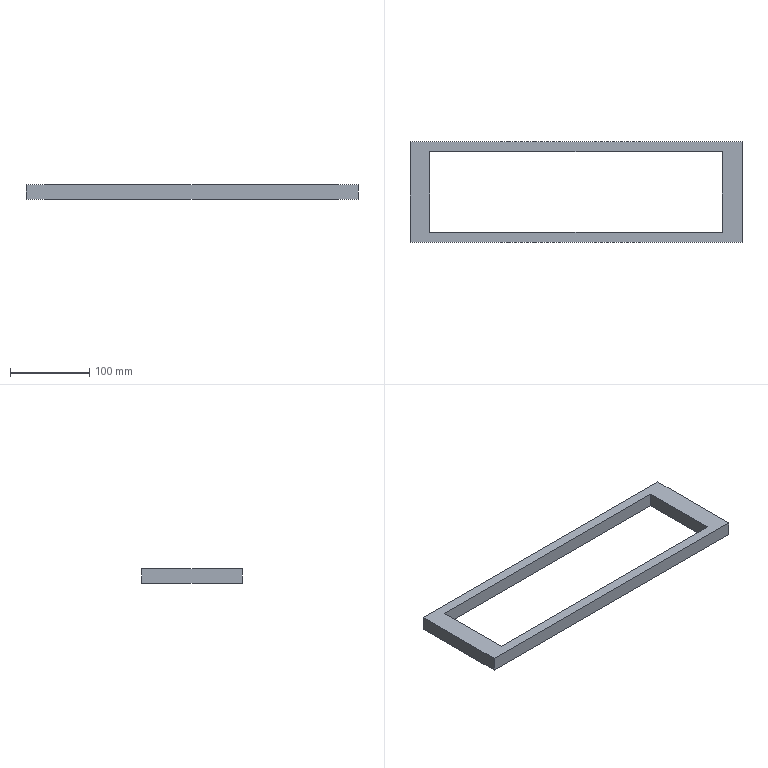Part | SolidWorks | features Extrusion 1 | 1 solid | 10 faces | box 420 x 127 x 18 mm | volume 280800 mm3 | plane 10
STEP:
#1=CARTESIAN_POINT('',(-210.,63.5,9.));
#2=VERTEX_POINT('',#1);
#3=CARTESIAN_POINT('',(-210.,-63.5,9.));
#4=VERTEX_POINT('',#3);
#5=CARTESIAN_POINT('',(-210.,63.5,9.));
#6=DIRECTION('',(0.,-1.,0.));
#7=VECTOR('',#6,1000.);
#8=LINE('',#5,#7);
#9=EDGE_CURVE('',#2,#4,#8,.T.);
#10=ORIENTED_EDGE('',*,*,#9,.F.);
#11=CARTESIAN_POINT('',(-210.,63.5,-9.));
#12=VERTEX_POINT('',#11);
#13=CARTESIAN_POINT('',(-210.,63.5,-9.));
#14=DIRECTION('',(0.,0.,1.));
#15=VECTOR('',#14,1000.);
#16=LINE('',#13,#15);
#17=EDGE_CURVE('',#12,#2,#16,.T.);
#18=ORIENTED_EDGE('',*,*,#17,.F.);
#19=CARTESIAN_POINT('',(-210.,-63.5,-9.));
#20=VERTEX_POINT('',#19);
#21=CARTESIAN_POINT('',(-210.,63.5,-9.));
#22=DIRECTION('',(0.,-1.,0.));
#23=VECTOR('',#22,1000.);
#24=LINE('',#21,#23);
#25=EDGE_CURVE('',#12,#20,#24,.T.);
#26=ORIENTED_EDGE('',*,*,#25,.T.);
#27=CARTESIAN_POINT('',(-210.,-63.5,-9.));
#28=DIRECTION('',(0.,0.,1.));
#29=VECTOR('',#28,1000.);
#30=LINE('',#27,#29);
#31=EDGE_CURVE('',#20,#4,#30,.T.);
#32=ORIENTED_EDGE('',*,*,#31,.T.);
#33=EDGE_LOOP('',(#10,#18,#26,#32));
#34=FACE_OUTER_BOUND('',#33,.T.);
#35=CARTESIAN_POINT('',(-210.,63.5,-9.));
#36=DIRECTION('',(-1.,0.,0.));
#37=DIRECTION('',(0.,0.,1.));
#38=AXIS2_PLACEMENT_3D('',#35,#36,#37);
#39=PLANE('',#38);
#40=ADVANCED_FACE('',(#34),#39,.T.);
#41=CARTESIAN_POINT('',(210.,63.5,9.));
#42=VERTEX_POINT('',#41);
#43=CARTESIAN_POINT('',(210.,63.5,9.));
#44=DIRECTION('',(-1.,0.,0.));
#45=VECTOR('',#44,1000.);
#46=LINE('',#43,#45);
#47=EDGE_CURVE('',#42,#2,#46,.T.);
#48=ORIENTED_EDGE('',*,*,#47,.F.);
#49=CARTESIAN_POINT('',(210.,63.5,-9.));
#50=VERTEX_POINT('',#49);
#51=CARTESIAN_POINT('',(210.,63.5,-9.));
#52=DIRECTION('',(0.,0.,1.));
#53=VECTOR('',#52,1000.);
#54=LINE('',#51,#53);
#55=EDGE_CURVE('',#50,#42,#54,.T.);
#56=ORIENTED_EDGE('',*,*,#55,.F.);
#57=CARTESIAN_POINT('',(210.,63.5,-9.));
#58=DIRECTION('',(-1.,0.,0.));
#59=VECTOR('',#58,1000.);
#60=LINE('',#57,#59);
#61=EDGE_CURVE('',#50,#12,#60,.T.);
#62=ORIENTED_EDGE('',*,*,#61,.T.);
#63=ORIENTED_EDGE('',*,*,#17,.T.);
#64=EDGE_LOOP('',(#48,#56,#62,#63));
#65=FACE_OUTER_BOUND('',#64,.T.);
#66=CARTESIAN_POINT('',(210.,63.5,-9.));
#67=DIRECTION('',(0.,1.,0.));
#68=DIRECTION('',(0.,0.,1.));
#69=AXIS2_PLACEMENT_3D('',#66,#67,#68);
#70=PLANE('',#69);
#71=ADVANCED_FACE('',(#65),#70,.T.);
#72=CARTESIAN_POINT('',(210.,-63.5,9.));
#73=VERTEX_POINT('',#72);
#74=CARTESIAN_POINT('',(210.,-63.5,9.));
#75=DIRECTION('',(0.,1.,0.));
#76=VECTOR('',#75,1000.);
#77=LINE('',#74,#76);
#78=EDGE_CURVE('',#73,#42,#77,.T.);
#79=ORIENTED_EDGE('',*,*,#78,.F.);
#80=CARTESIAN_POINT('',(210.,-63.5,-9.));
#81=VERTEX_POINT('',#80);
#82=CARTESIAN_POINT('',(210.,-63.5,-9.));
#83=DIRECTION('',(0.,0.,1.));
#84=VECTOR('',#83,1000.);
#85=LINE('',#82,#84);
#86=EDGE_CURVE('',#81,#73,#85,.T.);
#87=ORIENTED_EDGE('',*,*,#86,.F.);
#88=CARTESIAN_POINT('',(210.,-63.5,-9.));
#89=DIRECTION('',(0.,1.,0.));
#90=VECTOR('',#89,1000.);
#91=LINE('',#88,#90);
#92=EDGE_CURVE('',#81,#50,#91,.T.);
#93=ORIENTED_EDGE('',*,*,#92,.T.);
#94=ORIENTED_EDGE('',*,*,#55,.T.);
#95=EDGE_LOOP('',(#79,#87,#93,#94));
#96=FACE_OUTER_BOUND('',#95,.T.);
#97=CARTESIAN_POINT('',(210.,-63.5,-9.));
#98=DIRECTION('',(1.,0.,0.));
#99=DIRECTION('',(0.,0.,-1.));
#100=AXIS2_PLACEMENT_3D('',#97,#98,#99);
#101=PLANE('',#100);
#102=ADVANCED_FACE('',(#96),#101,.T.);
#103=CARTESIAN_POINT('',(-210.,-63.5,9.));
#104=DIRECTION('',(1.,0.,0.));
#105=VECTOR('',#104,1000.);
#106=LINE('',#103,#105);
#107=EDGE_CURVE('',#4,#73,#106,.T.);
#108=ORIENTED_EDGE('',*,*,#107,.F.);
#109=ORIENTED_EDGE('',*,*,#31,.F.);
#110=CARTESIAN_POINT('',(-210.,-63.5,-9.));
#111=DIRECTION('',(1.,0.,0.));
#112=VECTOR('',#111,1000.);
#113=LINE('',#110,#112);
#114=EDGE_CURVE('',#20,#81,#113,.T.);
#115=ORIENTED_EDGE('',*,*,#114,.T.);
#116=ORIENTED_EDGE('',*,*,#86,.T.);
#117=EDGE_LOOP('',(#108,#109,#115,#116));
#118=FACE_OUTER_BOUND('',#117,.T.);
#119=CARTESIAN_POINT('',(-210.,-63.5,-9.));
#120=DIRECTION('',(0.,-1.,0.));
#121=DIRECTION('',(0.,0.,-1.));
#122=AXIS2_PLACEMENT_3D('',#119,#120,#121);
#123=PLANE('',#122);
#124=ADVANCED_FACE('',(#118),#123,.T.);
#125=CARTESIAN_POINT('',(185.,51.,-9.));
#126=VERTEX_POINT('',#125);
#127=CARTESIAN_POINT('',(-185.,51.,-9.));
#128=VERTEX_POINT('',#127);
#129=CARTESIAN_POINT('',(185.,51.,-9.));
#130=DIRECTION('',(-1.,0.,0.));
#131=VECTOR('',#130,1000.);
#132=LINE('',#129,#131);
#133=EDGE_CURVE('',#126,#128,#132,.T.);
#134=ORIENTED_EDGE('',*,*,#133,.T.);
#135=CARTESIAN_POINT('',(-185.,-51.,-9.));
#136=VERTEX_POINT('',#135);
#137=CARTESIAN_POINT('',(-185.,51.,-9.));
#138=DIRECTION('',(0.,-1.,0.));
#139=VECTOR('',#138,1000.);
#140=LINE('',#137,#139);
#141=EDGE_CURVE('',#128,#136,#140,.T.);
#142=ORIENTED_EDGE('',*,*,#141,.T.);
#143=CARTESIAN_POINT('',(185.,-51.,-9.));
#144=VERTEX_POINT('',#143);
#145=CARTESIAN_POINT('',(-185.,-51.,-9.));
#146=DIRECTION('',(1.,0.,0.));
#147=VECTOR('',#146,1000.);
#148=LINE('',#145,#147);
#149=EDGE_CURVE('',#136,#144,#148,.T.);
#150=ORIENTED_EDGE('',*,*,#149,.T.);
#151=CARTESIAN_POINT('',(185.,-51.,-9.));
#152=DIRECTION('',(0.,1.,0.));
#153=VECTOR('',#152,1000.);
#154=LINE('',#151,#153);
#155=EDGE_CURVE('',#144,#126,#154,.T.);
#156=ORIENTED_EDGE('',*,*,#155,.T.);
#157=EDGE_LOOP('',(#134,#142,#150,#156));
#158=FACE_BOUND('',#157,.T.);
#159=ORIENTED_EDGE('',*,*,#25,.F.);
#160=ORIENTED_EDGE('',*,*,#61,.F.);
#161=ORIENTED_EDGE('',*,*,#92,.F.);
#162=ORIENTED_EDGE('',*,*,#114,.F.);
#163=EDGE_LOOP('',(#159,#160,#161,#162));
#164=FACE_OUTER_BOUND('',#163,.T.);
#165=CARTESIAN_POINT('',(0.,0.,-9.));
#166=DIRECTION('',(0.,0.,1.));
#167=DIRECTION('',(1.,0.,0.));
#168=AXIS2_PLACEMENT_3D('',#165,#166,#167);
#169=PLANE('',#168);
#170=ADVANCED_FACE('',(#158,#164),#169,.F.);
#171=CARTESIAN_POINT('',(-185.,51.,9.));
#172=VERTEX_POINT('',#171);
#173=CARTESIAN_POINT('',(-185.,-51.,9.));
#174=VERTEX_POINT('',#173);
#175=CARTESIAN_POINT('',(-185.,51.,9.));
#176=DIRECTION('',(0.,-1.,0.));
#177=VECTOR('',#176,1000.);
#178=LINE('',#175,#177);
#179=EDGE_CURVE('',#172,#174,#178,.T.);
#180=ORIENTED_EDGE('',*,*,#179,.F.);
#181=CARTESIAN_POINT('',(185.,51.,9.));
#182=VERTEX_POINT('',#181);
#183=CARTESIAN_POINT('',(185.,51.,9.));
#184=DIRECTION('',(-1.,0.,0.));
#185=VECTOR('',#184,1000.);
#186=LINE('',#183,#185);
#187=EDGE_CURVE('',#182,#172,#186,.T.);
#188=ORIENTED_EDGE('',*,*,#187,.F.);
#189=CARTESIAN_POINT('',(185.,-51.,9.));
#190=VERTEX_POINT('',#189);
#191=CARTESIAN_POINT('',(185.,-51.,9.));
#192=DIRECTION('',(0.,1.,0.));
#193=VECTOR('',#192,1000.);
#194=LINE('',#191,#193);
#195=EDGE_CURVE('',#190,#182,#194,.T.);
#196=ORIENTED_EDGE('',*,*,#195,.F.);
#197=CARTESIAN_POINT('',(-185.,-51.,9.));
#198=DIRECTION('',(1.,0.,0.));
#199=VECTOR('',#198,1000.);
#200=LINE('',#197,#199);
#201=EDGE_CURVE('',#174,#190,#200,.T.);
#202=ORIENTED_EDGE('',*,*,#201,.F.);
#203=EDGE_LOOP('',(#180,#188,#196,#202));
#204=FACE_BOUND('',#203,.T.);
#205=ORIENTED_EDGE('',*,*,#9,.T.);
#206=ORIENTED_EDGE('',*,*,#107,.T.);
#207=ORIENTED_EDGE('',*,*,#78,.T.);
#208=ORIENTED_EDGE('',*,*,#47,.T.);
#209=EDGE_LOOP('',(#205,#206,#207,#208));
#210=FACE_OUTER_BOUND('',#209,.T.);
#211=CARTESIAN_POINT('',(0.,0.,9.));
#212=DIRECTION('',(0.,0.,1.));
#213=DIRECTION('',(1.,0.,0.));
#214=AXIS2_PLACEMENT_3D('',#211,#212,#213);
#215=PLANE('',#214);
#216=ADVANCED_FACE('',(#204,#210),#215,.T.);
#217=ORIENTED_EDGE('',*,*,#179,.T.);
#218=CARTESIAN_POINT('',(-185.,-51.,-9.));
#219=DIRECTION('',(0.,0.,1.));
#220=VECTOR('',#219,1000.);
#221=LINE('',#218,#220);
#222=EDGE_CURVE('',#136,#174,#221,.T.);
#223=ORIENTED_EDGE('',*,*,#222,.F.);
#224=ORIENTED_EDGE('',*,*,#141,.F.);
#225=CARTESIAN_POINT('',(-185.,51.,-9.));
#226=DIRECTION('',(0.,0.,1.));
#227=VECTOR('',#226,1000.);
#228=LINE('',#225,#227);
#229=EDGE_CURVE('',#128,#172,#228,.T.);
#230=ORIENTED_EDGE('',*,*,#229,.T.);
#231=EDGE_LOOP('',(#217,#223,#224,#230));
#232=FACE_OUTER_BOUND('',#231,.T.);
#233=CARTESIAN_POINT('',(-185.,51.,-9.));
#234=DIRECTION('',(-1.,0.,0.));
#235=DIRECTION('',(0.,0.,1.));
#236=AXIS2_PLACEMENT_3D('',#233,#234,#235);
#237=PLANE('',#236);
#238=ADVANCED_FACE('',(#232),#237,.F.);
#239=ORIENTED_EDGE('',*,*,#187,.T.);
#240=ORIENTED_EDGE('',*,*,#229,.F.);
#241=ORIENTED_EDGE('',*,*,#133,.F.);
#242=CARTESIAN_POINT('',(185.,51.,-9.));
#243=DIRECTION('',(0.,0.,1.));
#244=VECTOR('',#243,1000.);
#245=LINE('',#242,#244);
#246=EDGE_CURVE('',#126,#182,#245,.T.);
#247=ORIENTED_EDGE('',*,*,#246,.T.);
#248=EDGE_LOOP('',(#239,#240,#241,#247));
#249=FACE_OUTER_BOUND('',#248,.T.);
#250=CARTESIAN_POINT('',(185.,51.,-9.));
#251=DIRECTION('',(0.,1.,0.));
#252=DIRECTION('',(0.,0.,1.));
#253=AXIS2_PLACEMENT_3D('',#250,#251,#252);
#254=PLANE('',#253);
#255=ADVANCED_FACE('',(#249),#254,.F.);
#256=ORIENTED_EDGE('',*,*,#195,.T.);
#257=ORIENTED_EDGE('',*,*,#246,.F.);
#258=ORIENTED_EDGE('',*,*,#155,.F.);
#259=CARTESIAN_POINT('',(185.,-51.,-9.));
#260=DIRECTION('',(0.,0.,1.));
#261=VECTOR('',#260,1000.);
#262=LINE('',#259,#261);
#263=EDGE_CURVE('',#144,#190,#262,.T.);
#264=ORIENTED_EDGE('',*,*,#263,.T.);
#265=EDGE_LOOP('',(#256,#257,#258,#264));
#266=FACE_OUTER_BOUND('',#265,.T.);
#267=CARTESIAN_POINT('',(185.,-51.,-9.));
#268=DIRECTION('',(1.,0.,0.));
#269=DIRECTION('',(0.,0.,-1.));
#270=AXIS2_PLACEMENT_3D('',#267,#268,#269);
#271=PLANE('',#270);
#272=ADVANCED_FACE('',(#266),#271,.F.);
#273=ORIENTED_EDGE('',*,*,#201,.T.);
#274=ORIENTED_EDGE('',*,*,#263,.F.);
#275=ORIENTED_EDGE('',*,*,#149,.F.);
#276=ORIENTED_EDGE('',*,*,#222,.T.);
#277=EDGE_LOOP('',(#273,#274,#275,#276));
#278=FACE_OUTER_BOUND('',#277,.T.);
#279=CARTESIAN_POINT('',(-185.,-51.,-9.));
#280=DIRECTION('',(0.,-1.,0.));
#281=DIRECTION('',(0.,0.,-1.));
#282=AXIS2_PLACEMENT_3D('',#279,#280,#281);
#283=PLANE('',#282);
#284=ADVANCED_FACE('',(#278),#283,.F.);
#285=CLOSED_SHELL('',(#40,#71,#102,#124,#170,#216,#238,#255,#272,#284));
#286=MANIFOLD_SOLID_BREP('',#285);
#287=CARTESIAN_POINT('',(0.,0.,0.));
#288=DIRECTION('',(0.,0.,1.));
#289=DIRECTION('',(1.,0.,0.));
#290=AXIS2_PLACEMENT_3D('',#287,#288,#289);
#291=(LENGTH_UNIT()NAMED_UNIT(*)SI_UNIT(.MILLI.,.METRE.));
#292=UNCERTAINTY_MEASURE_WITH_UNIT(LENGTH_MEASURE(0.00001),#291,'','');
#293=(NAMED_UNIT(*)PLANE_ANGLE_UNIT()SI_UNIT($,.RADIAN.));
#294=(NAMED_UNIT(*)SI_UNIT($,.STERADIAN.)SOLID_ANGLE_UNIT());
#295=(GEOMETRIC_REPRESENTATION_CONTEXT(3)GLOBAL_UNCERTAINTY_ASSIGNED_CONTEXT((#292))GLOBAL_UNIT_ASSIGNED_CONTEXT((#291,#293,#294))REPRESENTATION_CONTEXT('',''));
#296=ADVANCED_BREP_SHAPE_REPRESENTATION('',(#286,#290),#295);